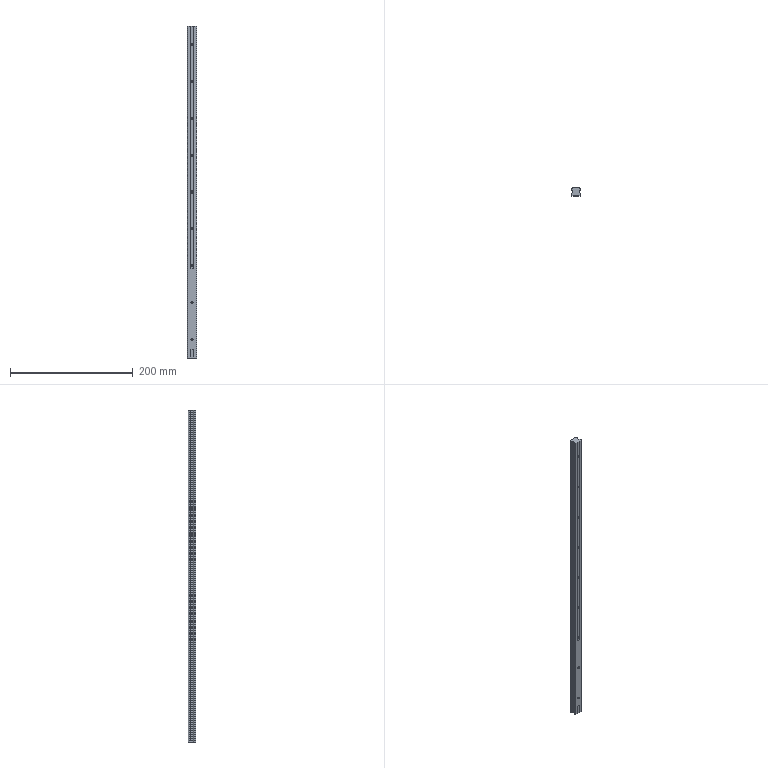Part | SolidWorks | features BaseBody 1, HoleWzd 1, ICE 1, MoveFace 1 | 1 solid | 87 faces | box 15 x 12.5 x 540 mm | volume 86755 mm3 | cylinder 54 | plane 33 | commonest cylinder face diameters 3.4 x18 6 x18 0.6 x11 3 x5 1 x2